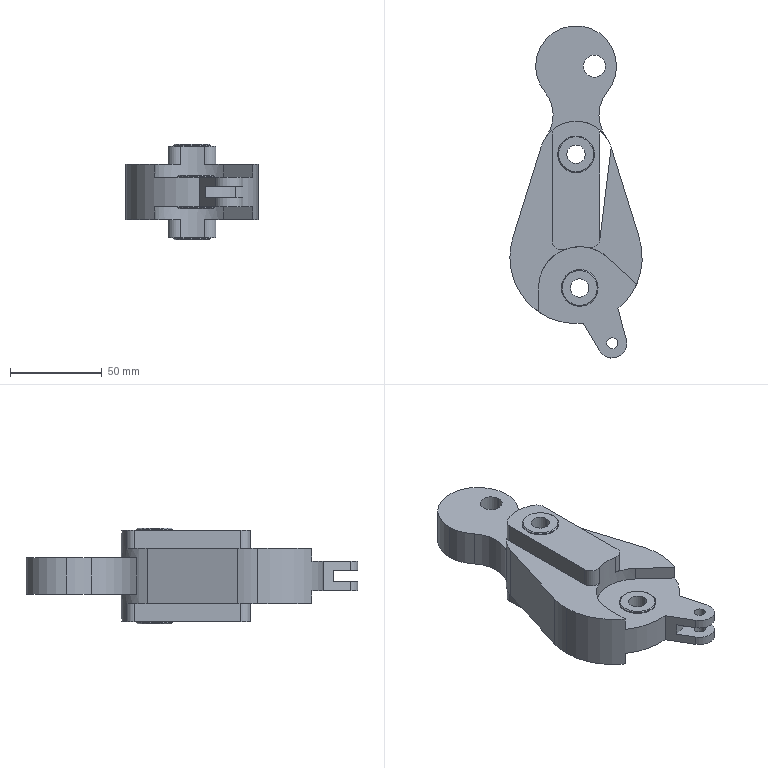Part | SolidWorks | features ICE 9, Chamfer 2, MirrorPattern 2, Extrusion 1 | 1 solid | 77 faces | box 72 x 180.817 x 52 mm | volume 220278 mm3 | cylinder 41 | plane 28 | cone 8 | commonest cylinder face diameters 10 x12 20 x8 6 x4 40 x4 44 x3 72 x3